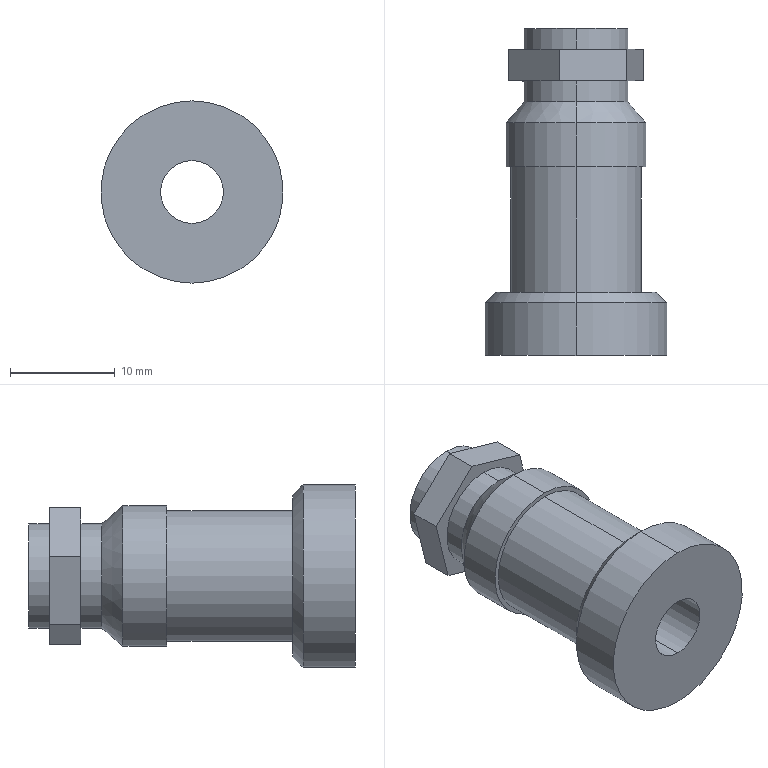Part | SolidWorks | features ICE 2, Chamfer 1, Revolution 1 | 1 solid | 28 faces | box 17.4 x 31.2 x 17.4 mm | volume 3464 mm3 | cylinder 12 | plane 12 | cone 4 | commonest cylinder face diameters 10 x4 6 x2 12.5 x2 13.4 x2 17.4 x2
STEP:
#1=CARTESIAN_POINT('',(0.,-25.2,7.7));
#2=VERTEX_POINT('',#1);
#3=CARTESIAN_POINT('',(0.,-25.2,-7.7));
#4=VERTEX_POINT('',#3);
#5=CARTESIAN_POINT('',(0.,-25.2,0.));
#6=DIRECTION('',(0.,1.,0.));
#7=DIRECTION('',(0.,0.,-1.));
#8=AXIS2_PLACEMENT_3D('',#5,#6,#7);
#9=CIRCLE('',#8,7.7);
#10=EDGE_CURVE('',#2,#4,#9,.T.);
#11=ORIENTED_EDGE('',*,*,#10,.F.);
#12=CARTESIAN_POINT('',(0.,-26.2,8.7));
#13=VERTEX_POINT('',#12);
#14=CARTESIAN_POINT('',(0.,-25.2,7.7));
#15=DIRECTION('',(0.,-0.7071,0.7071));
#16=VECTOR('',#15,1000.);
#17=LINE('',#14,#16);
#18=EDGE_CURVE('',#2,#13,#17,.T.);
#19=ORIENTED_EDGE('',*,*,#18,.T.);
#20=CARTESIAN_POINT('',(0.,-26.2,-8.7));
#21=VERTEX_POINT('',#20);
#22=CARTESIAN_POINT('',(0.,-26.2,0.));
#23=DIRECTION('',(0.,-1.,0.));
#24=DIRECTION('',(0.,0.,-1.));
#25=AXIS2_PLACEMENT_3D('',#22,#23,#24);
#26=CIRCLE('',#25,8.7);
#27=EDGE_CURVE('',#21,#13,#26,.T.);
#28=ORIENTED_EDGE('',*,*,#27,.F.);
#29=CARTESIAN_POINT('',(0.,-25.2,-7.7));
#30=DIRECTION('',(0.,-0.7071,-0.7071));
#31=VECTOR('',#30,1000.);
#32=LINE('',#29,#31);
#33=EDGE_CURVE('',#4,#21,#32,.T.);
#34=ORIENTED_EDGE('',*,*,#33,.F.);
#35=EDGE_LOOP('',(#11,#19,#28,#34));
#36=FACE_OUTER_BOUND('',#35,.T.);
#37=CARTESIAN_POINT('',(0.,-25.2,0.));
#38=DIRECTION('',(0.,-1.,0.));
#39=DIRECTION('',(0.,0.,-1.));
#40=AXIS2_PLACEMENT_3D('',#37,#38,#39);
#41=CONICAL_SURFACE('',#40,7.7,0.7854);
#42=ADVANCED_FACE('',(#36),#41,.T.);
#43=CARTESIAN_POINT('',(0.,-31.2,-3.));
#44=VERTEX_POINT('',#43);
#45=CARTESIAN_POINT('',(0.,-31.2,3.));
#46=VERTEX_POINT('',#45);
#47=CARTESIAN_POINT('',(0.,-31.2,0.));
#48=DIRECTION('',(0.,1.,0.));
#49=DIRECTION('',(0.,0.,1.));
#50=AXIS2_PLACEMENT_3D('',#47,#48,#49);
#51=CIRCLE('',#50,3.);
#52=EDGE_CURVE('',#44,#46,#51,.T.);
#53=ORIENTED_EDGE('',*,*,#52,.F.);
#54=CARTESIAN_POINT('',(0.,0.,-3.));
#55=VERTEX_POINT('',#54);
#56=CARTESIAN_POINT('',(0.,-31.2,-3.));
#57=DIRECTION('',(0.,1.,0.));
#58=VECTOR('',#57,1000.);
#59=LINE('',#56,#58);
#60=EDGE_CURVE('',#44,#55,#59,.T.);
#61=ORIENTED_EDGE('',*,*,#60,.T.);
#62=CARTESIAN_POINT('',(0.,0.,3.));
#63=VERTEX_POINT('',#62);
#64=CARTESIAN_POINT('',(0.,0.,0.));
#65=DIRECTION('',(0.,1.,0.));
#66=DIRECTION('',(0.,0.,1.));
#67=AXIS2_PLACEMENT_3D('',#64,#65,#66);
#68=CIRCLE('',#67,3.);
#69=EDGE_CURVE('',#55,#63,#68,.T.);
#70=ORIENTED_EDGE('',*,*,#69,.T.);
#71=CARTESIAN_POINT('',(0.,-31.2,3.));
#72=DIRECTION('',(0.,1.,0.));
#73=VECTOR('',#72,1000.);
#74=LINE('',#71,#73);
#75=EDGE_CURVE('',#46,#63,#74,.T.);
#76=ORIENTED_EDGE('',*,*,#75,.F.);
#77=EDGE_LOOP('',(#53,#61,#70,#76));
#78=FACE_OUTER_BOUND('',#77,.T.);
#79=CARTESIAN_POINT('',(0.,-31.2,0.));
#80=DIRECTION('',(0.,1.,0.));
#81=DIRECTION('',(0.,0.,1.));
#82=AXIS2_PLACEMENT_3D('',#79,#80,#81);
#83=CYLINDRICAL_SURFACE('',#82,3.);
#84=ADVANCED_FACE('',(#78),#83,.F.);
#85=CARTESIAN_POINT('',(0.,-2.,5.));
#86=VERTEX_POINT('',#85);
#87=CARTESIAN_POINT('',(0.,-2.,-5.));
#88=VERTEX_POINT('',#87);
#89=CARTESIAN_POINT('',(0.,-2.,0.));
#90=DIRECTION('',(0.,1.,0.));
#91=DIRECTION('',(0.,0.,1.));
#92=AXIS2_PLACEMENT_3D('',#89,#90,#91);
#93=CIRCLE('',#92,5.);
#94=EDGE_CURVE('',#86,#88,#93,.T.);
#95=ORIENTED_EDGE('',*,*,#94,.T.);
#96=CARTESIAN_POINT('',(0.,0.,-5.));
#97=VERTEX_POINT('',#96);
#98=CARTESIAN_POINT('',(0.,0.,-5.));
#99=DIRECTION('',(0.,1.,0.));
#100=VECTOR('',#99,1000.);
#101=LINE('',#98,#100);
#102=EDGE_CURVE('',#88,#97,#101,.T.);
#103=ORIENTED_EDGE('',*,*,#102,.T.);
#104=CARTESIAN_POINT('',(0.,0.,5.));
#105=VERTEX_POINT('',#104);
#106=CARTESIAN_POINT('',(0.,0.,0.));
#107=DIRECTION('',(0.,1.,0.));
#108=DIRECTION('',(0.,0.,1.));
#109=AXIS2_PLACEMENT_3D('',#106,#107,#108);
#110=CIRCLE('',#109,5.);
#111=EDGE_CURVE('',#105,#97,#110,.T.);
#112=ORIENTED_EDGE('',*,*,#111,.F.);
#113=CARTESIAN_POINT('',(0.,0.,5.));
#114=DIRECTION('',(0.,1.,0.));
#115=VECTOR('',#114,1000.);
#116=LINE('',#113,#115);
#117=EDGE_CURVE('',#86,#105,#116,.T.);
#118=ORIENTED_EDGE('',*,*,#117,.F.);
#119=EDGE_LOOP('',(#95,#103,#112,#118));
#120=FACE_OUTER_BOUND('',#119,.T.);
#121=CARTESIAN_POINT('',(0.,0.,0.));
#122=DIRECTION('',(0.,1.,0.));
#123=DIRECTION('',(0.,0.,1.));
#124=AXIS2_PLACEMENT_3D('',#121,#122,#123);
#125=CYLINDRICAL_SURFACE('',#124,5.);
#126=ADVANCED_FACE('',(#120),#125,.T.);
#127=CARTESIAN_POINT('',(0.,-31.2,8.7));
#128=VERTEX_POINT('',#127);
#129=CARTESIAN_POINT('',(0.,-31.2,-8.7));
#130=VERTEX_POINT('',#129);
#131=CARTESIAN_POINT('',(0.,-31.2,0.));
#132=DIRECTION('',(0.,1.,0.));
#133=DIRECTION('',(0.,0.,1.));
#134=AXIS2_PLACEMENT_3D('',#131,#132,#133);
#135=CIRCLE('',#134,8.7);
#136=EDGE_CURVE('',#128,#130,#135,.T.);
#137=ORIENTED_EDGE('',*,*,#136,.T.);
#138=CARTESIAN_POINT('',(0.,0.,-8.7));
#139=DIRECTION('',(0.,1.,0.));
#140=VECTOR('',#139,1000.);
#141=LINE('',#138,#140);
#142=EDGE_CURVE('',#130,#21,#141,.T.);
#143=ORIENTED_EDGE('',*,*,#142,.T.);
#144=ORIENTED_EDGE('',*,*,#27,.T.);
#145=CARTESIAN_POINT('',(0.,0.,8.7));
#146=DIRECTION('',(0.,1.,0.));
#147=VECTOR('',#146,1000.);
#148=LINE('',#145,#147);
#149=EDGE_CURVE('',#128,#13,#148,.T.);
#150=ORIENTED_EDGE('',*,*,#149,.F.);
#151=EDGE_LOOP('',(#137,#143,#144,#150));
#152=FACE_OUTER_BOUND('',#151,.T.);
#153=CARTESIAN_POINT('',(0.,0.,0.));
#154=DIRECTION('',(0.,1.,0.));
#155=DIRECTION('',(0.,0.,1.));
#156=AXIS2_PLACEMENT_3D('',#153,#154,#155);
#157=CYLINDRICAL_SURFACE('',#156,8.7);
#158=ADVANCED_FACE('',(#152),#157,.T.);
#159=CARTESIAN_POINT('',(0.,-25.2,6.25));
#160=VERTEX_POINT('',#159);
#161=CARTESIAN_POINT('',(0.,-25.2,-6.25));
#162=VERTEX_POINT('',#161);
#163=CARTESIAN_POINT('',(0.,-25.2,0.));
#164=DIRECTION('',(0.,1.,0.));
#165=DIRECTION('',(0.,0.,1.));
#166=AXIS2_PLACEMENT_3D('',#163,#164,#165);
#167=CIRCLE('',#166,6.25);
#168=EDGE_CURVE('',#160,#162,#167,.T.);
#169=ORIENTED_EDGE('',*,*,#168,.T.);
#170=CARTESIAN_POINT('',(0.,-13.2,-6.25));
#171=VERTEX_POINT('',#170);
#172=CARTESIAN_POINT('',(0.,0.,-6.25));
#173=DIRECTION('',(0.,1.,0.));
#174=VECTOR('',#173,1000.);
#175=LINE('',#172,#174);
#176=EDGE_CURVE('',#162,#171,#175,.T.);
#177=ORIENTED_EDGE('',*,*,#176,.T.);
#178=CARTESIAN_POINT('',(0.,-13.2,6.25));
#179=VERTEX_POINT('',#178);
#180=CARTESIAN_POINT('',(0.,-13.2,0.));
#181=DIRECTION('',(0.,1.,0.));
#182=DIRECTION('',(0.,0.,1.));
#183=AXIS2_PLACEMENT_3D('',#180,#181,#182);
#184=CIRCLE('',#183,6.25);
#185=EDGE_CURVE('',#179,#171,#184,.T.);
#186=ORIENTED_EDGE('',*,*,#185,.F.);
#187=CARTESIAN_POINT('',(0.,0.,6.25));
#188=DIRECTION('',(0.,1.,0.));
#189=VECTOR('',#188,1000.);
#190=LINE('',#187,#189);
#191=EDGE_CURVE('',#160,#179,#190,.T.);
#192=ORIENTED_EDGE('',*,*,#191,.F.);
#193=EDGE_LOOP('',(#169,#177,#186,#192));
#194=FACE_OUTER_BOUND('',#193,.T.);
#195=CARTESIAN_POINT('',(0.,0.,0.));
#196=DIRECTION('',(0.,1.,0.));
#197=DIRECTION('',(0.,0.,1.));
#198=AXIS2_PLACEMENT_3D('',#195,#196,#197);
#199=CYLINDRICAL_SURFACE('',#198,6.25);
#200=ADVANCED_FACE('',(#194),#199,.T.);
#201=CARTESIAN_POINT('',(0.,-13.2,6.7));
#202=VERTEX_POINT('',#201);
#203=CARTESIAN_POINT('',(0.,-13.2,-6.7));
#204=VERTEX_POINT('',#203);
#205=CARTESIAN_POINT('',(0.,-13.2,0.));
#206=DIRECTION('',(0.,1.,0.));
#207=DIRECTION('',(0.,0.,1.));
#208=AXIS2_PLACEMENT_3D('',#205,#206,#207);
#209=CIRCLE('',#208,6.7);
#210=EDGE_CURVE('',#202,#204,#209,.T.);
#211=ORIENTED_EDGE('',*,*,#210,.T.);
#212=CARTESIAN_POINT('',(0.,-9.,-6.7));
#213=VERTEX_POINT('',#212);
#214=CARTESIAN_POINT('',(0.,0.,-6.7));
#215=DIRECTION('',(0.,1.,0.));
#216=VECTOR('',#215,1000.);
#217=LINE('',#214,#216);
#218=EDGE_CURVE('',#204,#213,#217,.T.);
#219=ORIENTED_EDGE('',*,*,#218,.T.);
#220=CARTESIAN_POINT('',(0.,-9.,6.7));
#221=VERTEX_POINT('',#220);
#222=CARTESIAN_POINT('',(0.,-9.,0.));
#223=DIRECTION('',(0.,1.,0.));
#224=DIRECTION('',(0.,0.,1.));
#225=AXIS2_PLACEMENT_3D('',#222,#223,#224);
#226=CIRCLE('',#225,6.7);
#227=EDGE_CURVE('',#221,#213,#226,.T.);
#228=ORIENTED_EDGE('',*,*,#227,.F.);
#229=CARTESIAN_POINT('',(0.,0.,6.7));
#230=DIRECTION('',(0.,1.,0.));
#231=VECTOR('',#230,1000.);
#232=LINE('',#229,#231);
#233=EDGE_CURVE('',#202,#221,#232,.T.);
#234=ORIENTED_EDGE('',*,*,#233,.F.);
#235=EDGE_LOOP('',(#211,#219,#228,#234));
#236=FACE_OUTER_BOUND('',#235,.T.);
#237=CARTESIAN_POINT('',(0.,0.,0.));
#238=DIRECTION('',(0.,1.,0.));
#239=DIRECTION('',(0.,0.,1.));
#240=AXIS2_PLACEMENT_3D('',#237,#238,#239);
#241=CYLINDRICAL_SURFACE('',#240,6.7);
#242=ADVANCED_FACE('',(#236),#241,.T.);
#243=CARTESIAN_POINT('',(0.,-7.,5.));
#244=VERTEX_POINT('',#243);
#245=CARTESIAN_POINT('',(0.,-7.,-5.));
#246=VERTEX_POINT('',#245);
#247=CARTESIAN_POINT('',(0.,-7.,0.));
#248=DIRECTION('',(0.,1.,0.));
#249=DIRECTION('',(0.,0.,1.));
#250=AXIS2_PLACEMENT_3D('',#247,#248,#249);
#251=CIRCLE('',#250,5.);
#252=EDGE_CURVE('',#244,#246,#251,.T.);
#253=ORIENTED_EDGE('',*,*,#252,.F.);
#254=CARTESIAN_POINT('',(0.,-9.,6.7));
#255=DIRECTION('',(0.,-0.7619,0.6476));
#256=VECTOR('',#255,1000.);
#257=LINE('',#254,#256);
#258=EDGE_CURVE('',#244,#221,#257,.T.);
#259=ORIENTED_EDGE('',*,*,#258,.T.);
#260=ORIENTED_EDGE('',*,*,#227,.T.);
#261=CARTESIAN_POINT('',(0.,-9.,-6.7));
#262=DIRECTION('',(0.,-0.7619,-0.6476));
#263=VECTOR('',#262,1000.);
#264=LINE('',#261,#263);
#265=EDGE_CURVE('',#246,#213,#264,.T.);
#266=ORIENTED_EDGE('',*,*,#265,.F.);
#267=EDGE_LOOP('',(#253,#259,#260,#266));
#268=FACE_OUTER_BOUND('',#267,.T.);
#269=CARTESIAN_POINT('',(0.,-9.,0.));
#270=DIRECTION('',(0.,-1.,0.));
#271=DIRECTION('',(0.,0.,-1.));
#272=AXIS2_PLACEMENT_3D('',#269,#270,#271);
#273=CONICAL_SURFACE('',#272,6.7,0.7045);
#274=ADVANCED_FACE('',(#268),#273,.T.);
#275=ORIENTED_EDGE('',*,*,#252,.T.);
#276=CARTESIAN_POINT('',(0.,-5.,-5.));
#277=VERTEX_POINT('',#276);
#278=CARTESIAN_POINT('',(0.,0.,-5.));
#279=DIRECTION('',(0.,1.,0.));
#280=VECTOR('',#279,1000.);
#281=LINE('',#278,#280);
#282=EDGE_CURVE('',#246,#277,#281,.T.);
#283=ORIENTED_EDGE('',*,*,#282,.T.);
#284=CARTESIAN_POINT('',(0.,-5.,5.));
#285=VERTEX_POINT('',#284);
#286=CARTESIAN_POINT('',(0.,-5.,0.));
#287=DIRECTION('',(0.,1.,0.));
#288=DIRECTION('',(0.,0.,1.));
#289=AXIS2_PLACEMENT_3D('',#286,#287,#288);
#290=CIRCLE('',#289,5.);
#291=EDGE_CURVE('',#285,#277,#290,.T.);
#292=ORIENTED_EDGE('',*,*,#291,.F.);
#293=CARTESIAN_POINT('',(0.,0.,5.));
#294=DIRECTION('',(0.,1.,0.));
#295=VECTOR('',#294,1000.);
#296=LINE('',#293,#295);
#297=EDGE_CURVE('',#244,#285,#296,.T.);
#298=ORIENTED_EDGE('',*,*,#297,.F.);
#299=EDGE_LOOP('',(#275,#283,#292,#298));
#300=FACE_OUTER_BOUND('',#299,.T.);
#301=CARTESIAN_POINT('',(0.,0.,0.));
#302=DIRECTION('',(0.,1.,0.));
#303=DIRECTION('',(0.,0.,1.));
#304=AXIS2_PLACEMENT_3D('',#301,#302,#303);
#305=CYLINDRICAL_SURFACE('',#304,5.);
#306=ADVANCED_FACE('',(#300),#305,.T.);
#307=ORIENTED_EDGE('',*,*,#282,.F.);
#308=CARTESIAN_POINT('',(0.,-7.,0.));
#309=DIRECTION('',(0.,1.,0.));
#310=DIRECTION('',(0.,0.,1.));
#311=AXIS2_PLACEMENT_3D('',#308,#309,#310);
#312=CIRCLE('',#311,5.);
#313=EDGE_CURVE('',#246,#244,#312,.T.);
#314=ORIENTED_EDGE('',*,*,#313,.T.);
#315=ORIENTED_EDGE('',*,*,#297,.T.);
#316=CARTESIAN_POINT('',(0.,-5.,0.));
#317=DIRECTION('',(0.,1.,0.));
#318=DIRECTION('',(0.,0.,1.));
#319=AXIS2_PLACEMENT_3D('',#316,#317,#318);
#320=CIRCLE('',#319,5.);
#321=EDGE_CURVE('',#277,#285,#320,.T.);
#322=ORIENTED_EDGE('',*,*,#321,.F.);
#323=EDGE_LOOP('',(#307,#314,#315,#322));
#324=FACE_OUTER_BOUND('',#323,.T.);
#325=CARTESIAN_POINT('',(0.,0.,0.));
#326=DIRECTION('',(0.,1.,0.));
#327=DIRECTION('',(0.,0.,1.));
#328=AXIS2_PLACEMENT_3D('',#325,#326,#327);
#329=CYLINDRICAL_SURFACE('',#328,5.);
#330=ADVANCED_FACE('',(#324),#329,.T.);
#331=ORIENTED_EDGE('',*,*,#258,.F.);
#332=ORIENTED_EDGE('',*,*,#313,.F.);
#333=ORIENTED_EDGE('',*,*,#265,.T.);
#334=CARTESIAN_POINT('',(0.,-9.,0.));
#335=DIRECTION('',(0.,1.,0.));
#336=DIRECTION('',(0.,0.,1.));
#337=AXIS2_PLACEMENT_3D('',#334,#335,#336);
#338=CIRCLE('',#337,6.7);
#339=EDGE_CURVE('',#213,#221,#338,.T.);
#340=ORIENTED_EDGE('',*,*,#339,.T.);
#341=EDGE_LOOP('',(#331,#332,#333,#340));
#342=FACE_OUTER_BOUND('',#341,.T.);
#343=CARTESIAN_POINT('',(0.,-9.,0.));
#344=DIRECTION('',(0.,-1.,0.));
#345=DIRECTION('',(0.,0.,-1.));
#346=AXIS2_PLACEMENT_3D('',#343,#344,#345);
#347=CONICAL_SURFACE('',#346,6.7,0.7045);
#348=ADVANCED_FACE('',(#342),#347,.T.);
#349=ORIENTED_EDGE('',*,*,#218,.F.);
#350=CARTESIAN_POINT('',(0.,-13.2,0.));
#351=DIRECTION('',(0.,1.,0.));
#352=DIRECTION('',(0.,0.,1.));
#353=AXIS2_PLACEMENT_3D('',#350,#351,#352);
#354=CIRCLE('',#353,6.7);
#355=EDGE_CURVE('',#204,#202,#354,.T.);
#356=ORIENTED_EDGE('',*,*,#355,.T.);
#357=ORIENTED_EDGE('',*,*,#233,.T.);
#358=ORIENTED_EDGE('',*,*,#339,.F.);
#359=EDGE_LOOP('',(#349,#356,#357,#358));
#360=FACE_OUTER_BOUND('',#359,.T.);
#361=CARTESIAN_POINT('',(0.,0.,0.));
#362=DIRECTION('',(0.,1.,0.));
#363=DIRECTION('',(0.,0.,1.));
#364=AXIS2_PLACEMENT_3D('',#361,#362,#363);
#365=CYLINDRICAL_SURFACE('',#364,6.7);
#366=ADVANCED_FACE('',(#360),#365,.T.);
#367=ORIENTED_EDGE('',*,*,#210,.F.);
#368=ORIENTED_EDGE('',*,*,#355,.F.);
#369=EDGE_LOOP('',(#367,#368));
#370=FACE_OUTER_BOUND('',#369,.T.);
#371=ORIENTED_EDGE('',*,*,#185,.T.);
#372=CARTESIAN_POINT('',(0.,-13.2,0.));
#373=DIRECTION('',(0.,1.,0.));
#374=DIRECTION('',(0.,0.,1.));
#375=AXIS2_PLACEMENT_3D('',#372,#373,#374);
#376=CIRCLE('',#375,6.25);
#377=EDGE_CURVE('',#171,#179,#376,.T.);
#378=ORIENTED_EDGE('',*,*,#377,.T.);
#379=EDGE_LOOP('',(#371,#378));
#380=FACE_BOUND('',#379,.T.);
#381=CARTESIAN_POINT('',(6.7,-13.2,0.));
#382=DIRECTION('',(0.,1.,0.));
#383=DIRECTION('',(0.,0.,1.));
#384=AXIS2_PLACEMENT_3D('',#381,#382,#383);
#385=PLANE('',#384);
#386=ADVANCED_FACE('',(#370,#380),#385,.F.);
#387=ORIENTED_EDGE('',*,*,#176,.F.);
#388=CARTESIAN_POINT('',(0.,-25.2,0.));
#389=DIRECTION('',(0.,1.,0.));
#390=DIRECTION('',(0.,0.,1.));
#391=AXIS2_PLACEMENT_3D('',#388,#389,#390);
#392=CIRCLE('',#391,6.25);
#393=EDGE_CURVE('',#162,#160,#392,.T.);
#394=ORIENTED_EDGE('',*,*,#393,.T.);
#395=ORIENTED_EDGE('',*,*,#191,.T.);
#396=ORIENTED_EDGE('',*,*,#377,.F.);
#397=EDGE_LOOP('',(#387,#394,#395,#396));
#398=FACE_OUTER_BOUND('',#397,.T.);
#399=CARTESIAN_POINT('',(0.,0.,0.));
#400=DIRECTION('',(0.,1.,0.));
#401=DIRECTION('',(0.,0.,1.));
#402=AXIS2_PLACEMENT_3D('',#399,#400,#401);
#403=CYLINDRICAL_SURFACE('',#402,6.25);
#404=ADVANCED_FACE('',(#398),#403,.T.);
#405=CARTESIAN_POINT('',(0.,-25.2,0.));
#406=DIRECTION('',(0.,1.,0.));
#407=DIRECTION('',(0.,0.,-1.));
#408=AXIS2_PLACEMENT_3D('',#405,#406,#407);
#409=CIRCLE('',#408,7.7);
#410=EDGE_CURVE('',#4,#2,#409,.T.);
#411=ORIENTED_EDGE('',*,*,#410,.T.);
#412=ORIENTED_EDGE('',*,*,#10,.T.);
#413=EDGE_LOOP('',(#411,#412));
#414=FACE_OUTER_BOUND('',#413,.T.);
#415=ORIENTED_EDGE('',*,*,#168,.F.);
#416=ORIENTED_EDGE('',*,*,#393,.F.);
#417=EDGE_LOOP('',(#415,#416));
#418=FACE_BOUND('',#417,.T.);
#419=CARTESIAN_POINT('',(6.25,-25.2,0.));
#420=DIRECTION('',(0.,-1.,0.));
#421=DIRECTION('',(0.,0.,-1.));
#422=AXIS2_PLACEMENT_3D('',#419,#420,#421);
#423=PLANE('',#422);
#424=ADVANCED_FACE('',(#414,#418),#423,.F.);
#425=ORIENTED_EDGE('',*,*,#142,.F.);
#426=CARTESIAN_POINT('',(0.,-31.2,0.));
#427=DIRECTION('',(0.,1.,0.));
#428=DIRECTION('',(0.,0.,1.));
#429=AXIS2_PLACEMENT_3D('',#426,#427,#428);
#430=CIRCLE('',#429,8.7);
#431=EDGE_CURVE('',#130,#128,#430,.T.);
#432=ORIENTED_EDGE('',*,*,#431,.T.);
#433=ORIENTED_EDGE('',*,*,#149,.T.);
#434=CARTESIAN_POINT('',(0.,-26.2,0.));
#435=DIRECTION('',(0.,-1.,0.));
#436=DIRECTION('',(0.,0.,-1.));
#437=AXIS2_PLACEMENT_3D('',#434,#435,#436);
#438=CIRCLE('',#437,8.7);
#439=EDGE_CURVE('',#13,#21,#438,.T.);
#440=ORIENTED_EDGE('',*,*,#439,.T.);
#441=EDGE_LOOP('',(#425,#432,#433,#440));
#442=FACE_OUTER_BOUND('',#441,.T.);
#443=CARTESIAN_POINT('',(0.,0.,0.));
#444=DIRECTION('',(0.,1.,0.));
#445=DIRECTION('',(0.,0.,1.));
#446=AXIS2_PLACEMENT_3D('',#443,#444,#445);
#447=CYLINDRICAL_SURFACE('',#446,8.7);
#448=ADVANCED_FACE('',(#442),#447,.T.);
#449=CARTESIAN_POINT('',(0.,-31.2,0.));
#450=DIRECTION('',(0.,1.,0.));
#451=DIRECTION('',(0.,0.,1.));
#452=AXIS2_PLACEMENT_3D('',#449,#450,#451);
#453=CIRCLE('',#452,3.);
#454=EDGE_CURVE('',#46,#44,#453,.T.);
#455=ORIENTED_EDGE('',*,*,#454,.T.);
#456=ORIENTED_EDGE('',*,*,#52,.T.);
#457=EDGE_LOOP('',(#455,#456));
#458=FACE_BOUND('',#457,.T.);
#459=ORIENTED_EDGE('',*,*,#136,.F.);
#460=ORIENTED_EDGE('',*,*,#431,.F.);
#461=EDGE_LOOP('',(#459,#460));
#462=FACE_OUTER_BOUND('',#461,.T.);
#463=CARTESIAN_POINT('',(8.7,-31.2,0.));
#464=DIRECTION('',(0.,1.,0.));
#465=DIRECTION('',(0.,0.,1.));
#466=AXIS2_PLACEMENT_3D('',#463,#464,#465);
#467=PLANE('',#466);
#468=ADVANCED_FACE('',(#458,#462),#467,.F.);
#469=CARTESIAN_POINT('',(-6.435,-2.,1.867));
#470=VERTEX_POINT('',#469);
#471=CARTESIAN_POINT('',(-1.6,-2.,6.506));
#472=VERTEX_POINT('',#471);
#473=CARTESIAN_POINT('',(-6.435,-2.,1.867));
#474=DIRECTION('',(0.7216,0.,0.6924));
#475=VECTOR('',#474,1000.);
#476=LINE('',#473,#475);
#477=EDGE_CURVE('',#470,#472,#476,.T.);
#478=ORIENTED_EDGE('',*,*,#477,.F.);
#479=CARTESIAN_POINT('',(-6.435,-5.,1.867));
#480=VERTEX_POINT('',#479);
#481=CARTESIAN_POINT('',(-6.435,-5.,1.867));
#482=DIRECTION('',(0.,1.,0.));
#483=VECTOR('',#482,1000.);
#484=LINE('',#481,#483);
#485=EDGE_CURVE('',#480,#470,#484,.T.);
#486=ORIENTED_EDGE('',*,*,#485,.F.);
#487=CARTESIAN_POINT('',(-1.6,-5.,6.506));
#488=VERTEX_POINT('',#487);
#489=CARTESIAN_POINT('',(-6.435,-5.,1.867));
#490=DIRECTION('',(0.7216,0.,0.6924));
#491=VECTOR('',#490,1000.);
#492=LINE('',#489,#491);
#493=EDGE_CURVE('',#480,#488,#492,.T.);
#494=ORIENTED_EDGE('',*,*,#493,.T.);
#495=CARTESIAN_POINT('',(-1.6,-5.,6.506));
#496=DIRECTION('',(0.,1.,0.));
#497=VECTOR('',#496,1000.);
#498=LINE('',#495,#497);
#499=EDGE_CURVE('',#488,#472,#498,.T.);
#500=ORIENTED_EDGE('',*,*,#499,.T.);
#501=EDGE_LOOP('',(#478,#486,#494,#500));
#502=FACE_OUTER_BOUND('',#501,.T.);
#503=CARTESIAN_POINT('',(-6.435,-5.,1.867));
#504=DIRECTION('',(-0.6924,0.,0.7216));
#505=DIRECTION('',(0.7216,0.,0.6924));
#506=AXIS2_PLACEMENT_3D('',#503,#504,#505);
#507=PLANE('',#506);
#508=ADVANCED_FACE('',(#502),#507,.T.);
#509=CARTESIAN_POINT('',(-4.834,-2.,-4.639));
#510=VERTEX_POINT('',#509);
#511=CARTESIAN_POINT('',(-4.834,-2.,-4.639));
#512=DIRECTION('',(-0.2388,0.,0.9711));
#513=VECTOR('',#512,1000.);
#514=LINE('',#511,#513);
#515=EDGE_CURVE('',#510,#470,#514,.T.);
#516=ORIENTED_EDGE('',*,*,#515,.F.);
#517=CARTESIAN_POINT('',(-4.834,-5.,-4.639));
#518=VERTEX_POINT('',#517);
#519=CARTESIAN_POINT('',(-4.834,-5.,-4.639));
#520=DIRECTION('',(0.,1.,0.));
#521=VECTOR('',#520,1000.);
#522=LINE('',#519,#521);
#523=EDGE_CURVE('',#518,#510,#522,.T.);
#524=ORIENTED_EDGE('',*,*,#523,.F.);
#525=CARTESIAN_POINT('',(-4.834,-5.,-4.639));
#526=DIRECTION('',(-0.2388,0.,0.9711));
#527=VECTOR('',#526,1000.);
#528=LINE('',#525,#527);
#529=EDGE_CURVE('',#518,#480,#528,.T.);
#530=ORIENTED_EDGE('',*,*,#529,.T.);
#531=ORIENTED_EDGE('',*,*,#485,.T.);
#532=EDGE_LOOP('',(#516,#524,#530,#531));
#533=FACE_OUTER_BOUND('',#532,.T.);
#534=CARTESIAN_POINT('',(-4.834,-5.,-4.639));
#535=DIRECTION('',(-0.9711,0.,-0.2388));
#536=DIRECTION('',(-0.2388,0.,0.9711));
#537=AXIS2_PLACEMENT_3D('',#534,#535,#536);
#538=PLANE('',#537);
#539=ADVANCED_FACE('',(#533),#538,.T.);
#540=CARTESIAN_POINT('',(1.6,-2.,-6.506));
#541=VERTEX_POINT('',#540);
#542=CARTESIAN_POINT('',(1.6,-2.,-6.506));
#543=DIRECTION('',(-0.9604,0.,0.2787));
#544=VECTOR('',#543,1000.);
#545=LINE('',#542,#544);
#546=EDGE_CURVE('',#541,#510,#545,.T.);
#547=ORIENTED_EDGE('',*,*,#546,.F.);
#548=CARTESIAN_POINT('',(1.6,-5.,-6.506));
#549=VERTEX_POINT('',#548);
#550=CARTESIAN_POINT('',(1.6,-5.,-6.506));
#551=DIRECTION('',(0.,1.,0.));
#552=VECTOR('',#551,1000.);
#553=LINE('',#550,#552);
#554=EDGE_CURVE('',#549,#541,#553,.T.);
#555=ORIENTED_EDGE('',*,*,#554,.F.);
#556=CARTESIAN_POINT('',(1.6,-5.,-6.506));
#557=DIRECTION('',(-0.9604,0.,0.2787));
#558=VECTOR('',#557,1000.);
#559=LINE('',#556,#558);
#560=EDGE_CURVE('',#549,#518,#559,.T.);
#561=ORIENTED_EDGE('',*,*,#560,.T.);
#562=ORIENTED_EDGE('',*,*,#523,.T.);
#563=EDGE_LOOP('',(#547,#555,#561,#562));
#564=FACE_OUTER_BOUND('',#563,.T.);
#565=CARTESIAN_POINT('',(1.6,-5.,-6.506));
#566=DIRECTION('',(-0.2787,0.,-0.9604));
#567=DIRECTION('',(-0.9604,0.,0.2787));
#568=AXIS2_PLACEMENT_3D('',#565,#566,#567);
#569=PLANE('',#568);
#570=ADVANCED_FACE('',(#564),#569,.T.);
#571=CARTESIAN_POINT('',(6.435,-2.,-1.867));
#572=VERTEX_POINT('',#571);
#573=CARTESIAN_POINT('',(6.435,-2.,-1.867));
#574=DIRECTION('',(-0.7216,0.,-0.6924));
#575=VECTOR('',#574,1000.);
#576=LINE('',#573,#575);
#577=EDGE_CURVE('',#572,#541,#576,.T.);
#578=ORIENTED_EDGE('',*,*,#577,.F.);
#579=CARTESIAN_POINT('',(6.435,-5.,-1.867));
#580=VERTEX_POINT('',#579);
#581=CARTESIAN_POINT('',(6.435,-5.,-1.867));
#582=DIRECTION('',(0.,1.,0.));
#583=VECTOR('',#582,1000.);
#584=LINE('',#581,#583);
#585=EDGE_CURVE('',#580,#572,#584,.T.);
#586=ORIENTED_EDGE('',*,*,#585,.F.);
#587=CARTESIAN_POINT('',(6.435,-5.,-1.867));
#588=DIRECTION('',(-0.7216,0.,-0.6924));
#589=VECTOR('',#588,1000.);
#590=LINE('',#587,#589);
#591=EDGE_CURVE('',#580,#549,#590,.T.);
#592=ORIENTED_EDGE('',*,*,#591,.T.);
#593=ORIENTED_EDGE('',*,*,#554,.T.);
#594=EDGE_LOOP('',(#578,#586,#592,#593));
#595=FACE_OUTER_BOUND('',#594,.T.);
#596=CARTESIAN_POINT('',(6.435,-5.,-1.867));
#597=DIRECTION('',(0.6924,0.,-0.7216));
#598=DIRECTION('',(-0.7216,0.,-0.6924));
#599=AXIS2_PLACEMENT_3D('',#596,#597,#598);
#600=PLANE('',#599);
#601=ADVANCED_FACE('',(#595),#600,.T.);
#602=CARTESIAN_POINT('',(4.834,-2.,4.639));
#603=VERTEX_POINT('',#602);
#604=CARTESIAN_POINT('',(4.834,-2.,4.639));
#605=DIRECTION('',(0.2388,0.,-0.9711));
#606=VECTOR('',#605,1000.);
#607=LINE('',#604,#606);
#608=EDGE_CURVE('',#603,#572,#607,.T.);
#609=ORIENTED_EDGE('',*,*,#608,.F.);
#610=CARTESIAN_POINT('',(4.834,-5.,4.639));
#611=VERTEX_POINT('',#610);
#612=CARTESIAN_POINT('',(4.834,-5.,4.639));
#613=DIRECTION('',(0.,1.,0.));
#614=VECTOR('',#613,1000.);
#615=LINE('',#612,#614);
#616=EDGE_CURVE('',#611,#603,#615,.T.);
#617=ORIENTED_EDGE('',*,*,#616,.F.);
#618=CARTESIAN_POINT('',(4.834,-5.,4.639));
#619=DIRECTION('',(0.2388,0.,-0.9711));
#620=VECTOR('',#619,1000.);
#621=LINE('',#618,#620);
#622=EDGE_CURVE('',#611,#580,#621,.T.);
#623=ORIENTED_EDGE('',*,*,#622,.T.);
#624=ORIENTED_EDGE('',*,*,#585,.T.);
#625=EDGE_LOOP('',(#609,#617,#623,#624));
#626=FACE_OUTER_BOUND('',#625,.T.);
#627=CARTESIAN_POINT('',(4.834,-5.,4.639));
#628=DIRECTION('',(0.9711,0.,0.2388));
#629=DIRECTION('',(0.2388,0.,-0.9711));
#630=AXIS2_PLACEMENT_3D('',#627,#628,#629);
#631=PLANE('',#630);
#632=ADVANCED_FACE('',(#626),#631,.T.);
#633=CARTESIAN_POINT('',(-1.6,-2.,6.506));
#634=DIRECTION('',(0.9604,0.,-0.2787));
#635=VECTOR('',#634,1000.);
#636=LINE('',#633,#635);
#637=EDGE_CURVE('',#472,#603,#636,.T.);
#638=ORIENTED_EDGE('',*,*,#637,.F.);
#639=ORIENTED_EDGE('',*,*,#499,.F.);
#640=CARTESIAN_POINT('',(-1.6,-5.,6.506));
#641=DIRECTION('',(0.9604,0.,-0.2787));
#642=VECTOR('',#641,1000.);
#643=LINE('',#640,#642);
#644=EDGE_CURVE('',#488,#611,#643,.T.);
#645=ORIENTED_EDGE('',*,*,#644,.T.);
#646=ORIENTED_EDGE('',*,*,#616,.T.);
#647=EDGE_LOOP('',(#638,#639,#645,#646));
#648=FACE_OUTER_BOUND('',#647,.T.);
#649=CARTESIAN_POINT('',(-1.6,-5.,6.506));
#650=DIRECTION('',(0.2787,0.,0.9604));
#651=DIRECTION('',(0.9604,0.,-0.2787));
#652=AXIS2_PLACEMENT_3D('',#649,#650,#651);
#653=PLANE('',#652);
#654=ADVANCED_FACE('',(#648),#653,.T.);
#655=ORIENTED_EDGE('',*,*,#291,.T.);
#656=ORIENTED_EDGE('',*,*,#321,.T.);
#657=EDGE_LOOP('',(#655,#656));
#658=FACE_BOUND('',#657,.T.);
#659=ORIENTED_EDGE('',*,*,#493,.F.);
#660=ORIENTED_EDGE('',*,*,#529,.F.);
#661=ORIENTED_EDGE('',*,*,#560,.F.);
#662=ORIENTED_EDGE('',*,*,#591,.F.);
#663=ORIENTED_EDGE('',*,*,#622,.F.);
#664=ORIENTED_EDGE('',*,*,#644,.F.);
#665=EDGE_LOOP('',(#659,#660,#661,#662,#663,#664));
#666=FACE_OUTER_BOUND('',#665,.T.);
#667=CARTESIAN_POINT('',(0.,-5.,0.));
#668=DIRECTION('',(0.,1.,0.));
#669=DIRECTION('',(0.,0.,1.));
#670=AXIS2_PLACEMENT_3D('',#667,#668,#669);
#671=PLANE('',#670);
#672=ADVANCED_FACE('',(#658,#666),#671,.F.);
#673=ORIENTED_EDGE('',*,*,#94,.F.);
#674=CARTESIAN_POINT('',(0.,-2.,0.));
#675=DIRECTION('',(0.,1.,0.));
#676=DIRECTION('',(0.,0.,1.));
#677=AXIS2_PLACEMENT_3D('',#674,#675,#676);
#678=CIRCLE('',#677,5.);
#679=EDGE_CURVE('',#88,#86,#678,.T.);
#680=ORIENTED_EDGE('',*,*,#679,.F.);
#681=EDGE_LOOP('',(#673,#680));
#682=FACE_BOUND('',#681,.T.);
#683=ORIENTED_EDGE('',*,*,#477,.T.);
#684=ORIENTED_EDGE('',*,*,#637,.T.);
#685=ORIENTED_EDGE('',*,*,#608,.T.);
#686=ORIENTED_EDGE('',*,*,#577,.T.);
#687=ORIENTED_EDGE('',*,*,#546,.T.);
#688=ORIENTED_EDGE('',*,*,#515,.T.);
#689=EDGE_LOOP('',(#683,#684,#685,#686,#687,#688));
#690=FACE_OUTER_BOUND('',#689,.T.);
#691=CARTESIAN_POINT('',(0.,-2.,0.));
#692=DIRECTION('',(0.,1.,0.));
#693=DIRECTION('',(0.,0.,1.));
#694=AXIS2_PLACEMENT_3D('',#691,#692,#693);
#695=PLANE('',#694);
#696=ADVANCED_FACE('',(#682,#690),#695,.T.);
#697=CARTESIAN_POINT('',(0.,0.,0.));
#698=DIRECTION('',(0.,1.,0.));
#699=DIRECTION('',(0.,0.,1.));
#700=AXIS2_PLACEMENT_3D('',#697,#698,#699);
#701=CIRCLE('',#700,3.);
#702=EDGE_CURVE('',#63,#55,#701,.T.);
#703=ORIENTED_EDGE('',*,*,#702,.F.);
#704=ORIENTED_EDGE('',*,*,#69,.F.);
#705=EDGE_LOOP('',(#703,#704));
#706=FACE_BOUND('',#705,.T.);
#707=ORIENTED_EDGE('',*,*,#111,.T.);
#708=CARTESIAN_POINT('',(0.,0.,0.));
#709=DIRECTION('',(0.,1.,0.));
#710=DIRECTION('',(0.,0.,1.));
#711=AXIS2_PLACEMENT_3D('',#708,#709,#710);
#712=CIRCLE('',#711,5.);
#713=EDGE_CURVE('',#97,#105,#712,.T.);
#714=ORIENTED_EDGE('',*,*,#713,.T.);
#715=EDGE_LOOP('',(#707,#714));
#716=FACE_OUTER_BOUND('',#715,.T.);
#717=CARTESIAN_POINT('',(0.,0.,0.));
#718=DIRECTION('',(0.,-1.,0.));
#719=DIRECTION('',(0.,0.,-1.));
#720=AXIS2_PLACEMENT_3D('',#717,#718,#719);
#721=PLANE('',#720);
#722=ADVANCED_FACE('',(#706,#716),#721,.F.);
#723=ORIENTED_EDGE('',*,*,#102,.F.);
#724=ORIENTED_EDGE('',*,*,#679,.T.);
#725=ORIENTED_EDGE('',*,*,#117,.T.);
#726=ORIENTED_EDGE('',*,*,#713,.F.);
#727=EDGE_LOOP('',(#723,#724,#725,#726));
#728=FACE_OUTER_BOUND('',#727,.T.);
#729=CARTESIAN_POINT('',(0.,0.,0.));
#730=DIRECTION('',(0.,1.,0.));
#731=DIRECTION('',(0.,0.,1.));
#732=AXIS2_PLACEMENT_3D('',#729,#730,#731);
#733=CYLINDRICAL_SURFACE('',#732,5.);
#734=ADVANCED_FACE('',(#728),#733,.T.);
#735=ORIENTED_EDGE('',*,*,#60,.F.);
#736=ORIENTED_EDGE('',*,*,#454,.F.);
#737=ORIENTED_EDGE('',*,*,#75,.T.);
#738=ORIENTED_EDGE('',*,*,#702,.T.);
#739=EDGE_LOOP('',(#735,#736,#737,#738));
#740=FACE_OUTER_BOUND('',#739,.T.);
#741=CARTESIAN_POINT('',(0.,-31.2,0.));
#742=DIRECTION('',(0.,1.,0.));
#743=DIRECTION('',(0.,0.,1.));
#744=AXIS2_PLACEMENT_3D('',#741,#742,#743);
#745=CYLINDRICAL_SURFACE('',#744,3.);
#746=ADVANCED_FACE('',(#740),#745,.F.);
#747=ORIENTED_EDGE('',*,*,#18,.F.);
#748=ORIENTED_EDGE('',*,*,#410,.F.);
#749=ORIENTED_EDGE('',*,*,#33,.T.);
#750=ORIENTED_EDGE('',*,*,#439,.F.);
#751=EDGE_LOOP('',(#747,#748,#749,#750));
#752=FACE_OUTER_BOUND('',#751,.T.);
#753=CARTESIAN_POINT('',(0.,-25.2,0.));
#754=DIRECTION('',(0.,-1.,0.));
#755=DIRECTION('',(0.,0.,-1.));
#756=AXIS2_PLACEMENT_3D('',#753,#754,#755);
#757=CONICAL_SURFACE('',#756,7.7,0.7854);
#758=ADVANCED_FACE('',(#752),#757,.T.);
#759=CLOSED_SHELL('',(#42,#84,#126,#158,#200,#242,#274,#306,#330,#348,#366,#386,#404,#424,#448,#468,#508,#539,#570,#601,#632,#654,#672,#696,#722,#734,#746,#758));
#760=MANIFOLD_SOLID_BREP('',#759);
#761=CARTESIAN_POINT('',(0.,0.,0.));
#762=DIRECTION('',(0.,0.,1.));
#763=DIRECTION('',(1.,0.,0.));
#764=AXIS2_PLACEMENT_3D('',#761,#762,#763);
#765=(LENGTH_UNIT()NAMED_UNIT(*)SI_UNIT(.MILLI.,.METRE.));
#766=UNCERTAINTY_MEASURE_WITH_UNIT(LENGTH_MEASURE(0.00001),#765,'','');
#767=(NAMED_UNIT(*)PLANE_ANGLE_UNIT()SI_UNIT($,.RADIAN.));
#768=(NAMED_UNIT(*)SI_UNIT($,.STERADIAN.)SOLID_ANGLE_UNIT());
#769=(GEOMETRIC_REPRESENTATION_CONTEXT(3)GLOBAL_UNCERTAINTY_ASSIGNED_CONTEXT((#766))GLOBAL_UNIT_ASSIGNED_CONTEXT((#765,#767,#768))REPRESENTATION_CONTEXT('',''));
#770=ADVANCED_BREP_SHAPE_REPRESENTATION('',(#760,#764),#769);